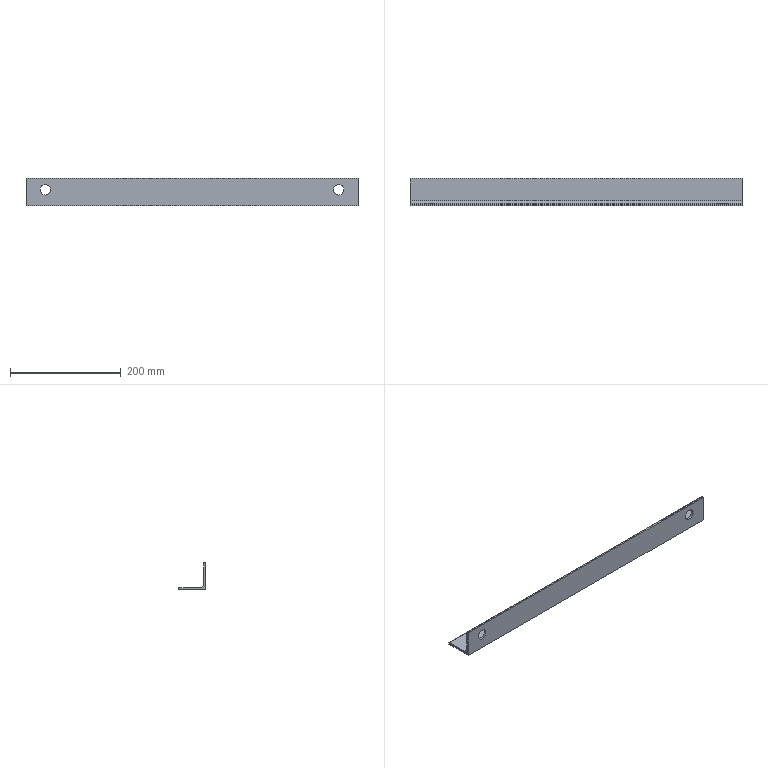Part | STEP file | 计量角钢3_Default<As Machined> | 1 solid | 15 faces | box 598.75 x 50 x 50 mm | volume 231084 mm3 | plane 8 | cylinder 7 | commonest cylinder face diameters 19 x4 2.66 x2 11 x1
STEP:
#1=CARTESIAN_POINT('',(0.,0.,0.));
#2=DIRECTION('',(0.,0.,1.));
#3=DIRECTION('',(1.,0.,0.));
#4=AXIS2_PLACEMENT_3D('',#1,#2,#3);
#5=CARTESIAN_POINT('',(-264.375,0.,38.585));
#6=VERTEX_POINT('',#5);
#7=CARTESIAN_POINT('',(-264.375,4.,38.585));
#8=VERTEX_POINT('',#7);
#9=CARTESIAN_POINT('',(-264.375,-6.,38.585));
#10=DIRECTION('',(0.,1.,0.));
#11=VECTOR('',#10,1.);
#12=LINE('',#9,#11);
#13=CARTESIAN_POINT('',(-264.375,-6.,29.085));
#14=DIRECTION('',(0.,1.,0.));
#15=DIRECTION('',(0.,0.,1.));
#16=AXIS2_PLACEMENT_3D('',#13,#14,#15);
#17=CYLINDRICAL_SURFACE('',#16,9.5);
#18=CARTESIAN_POINT('',(6.283,0.));
#19=DIRECTION('',(0.,1.));
#20=VECTOR('',#19,1.);
#21=LINE('',#18,#20);
#22=(GEOMETRIC_REPRESENTATION_CONTEXT(2)PARAMETRIC_REPRESENTATION_CONTEXT()REPRESENTATION_CONTEXT('',''));
#23=DEFINITIONAL_REPRESENTATION('',(#21),#22);
#24=PCURVE('',#17,#23);
#25=CARTESIAN_POINT('',(-264.375,-6.,29.085));
#26=DIRECTION('',(0.,1.,0.));
#27=DIRECTION('',(0.,0.,1.));
#28=AXIS2_PLACEMENT_3D('',#25,#26,#27);
#29=CYLINDRICAL_SURFACE('',#28,9.5);
#30=CARTESIAN_POINT('',(0.,0.));
#31=DIRECTION('',(0.,1.));
#32=VECTOR('',#31,1.);
#33=LINE('',#30,#32);
#34=(GEOMETRIC_REPRESENTATION_CONTEXT(2)PARAMETRIC_REPRESENTATION_CONTEXT()REPRESENTATION_CONTEXT('',''));
#35=DEFINITIONAL_REPRESENTATION('',(#33),#34);
#36=PCURVE('',#29,#35);
#37=SURFACE_CURVE('',#12,(#24,#36),.PCURVE_S1.);
#38=EDGE_CURVE('',#6,#8,#37,.T.);
#39=ORIENTED_EDGE('',*,*,#38,.T.);
#40=CARTESIAN_POINT('',(-264.375,4.,19.585));
#41=VERTEX_POINT('',#40);
#42=CARTESIAN_POINT('',(-264.375,4.,29.085));
#43=DIRECTION('',(0.,1.,0.));
#44=DIRECTION('',(0.,0.,1.));
#45=AXIS2_PLACEMENT_3D('',#42,#43,#44);
#46=CIRCLE('',#45,9.5);
#47=CARTESIAN_POINT('',(0.,10.));
#48=DIRECTION('',(1.,0.));
#49=VECTOR('',#48,1.);
#50=LINE('',#47,#49);
#51=(GEOMETRIC_REPRESENTATION_CONTEXT(2)PARAMETRIC_REPRESENTATION_CONTEXT()REPRESENTATION_CONTEXT('',''));
#52=DEFINITIONAL_REPRESENTATION('',(#50),#51);
#53=PCURVE('',#17,#52);
#54=CARTESIAN_POINT('',(299.375,4.,48.67));
#55=DIRECTION('',(0.,-1.,0.));
#56=DIRECTION('',(1.,0.,0.));
#57=AXIS2_PLACEMENT_3D('',#54,#55,#56);
#58=PLANE('',#57);
#59=CARTESIAN_POINT('',(-563.75,-10.085));
#60=CARTESIAN_POINT('',(-547.296,-10.085));
#61=CARTESIAN_POINT('',(-555.523,-24.335));
#62=CARTESIAN_POINT('',(-563.75,-38.585));
#63=CARTESIAN_POINT('',(-571.977,-24.335));
#64=CARTESIAN_POINT('',(-580.204,-10.085));
#65=CARTESIAN_POINT('',(-563.75,-10.085));
#66=(BOUNDED_CURVE()B_SPLINE_CURVE(2,(#59,#60,#61,#62,#63,#64,#65),.UNSPECIFIED.,.T.,.F.)B_SPLINE_CURVE_WITH_KNOTS((1,2,2,2,2,1),(-2.094,0.,2.094,4.189,6.283,8.378),.UNSPECIFIED.)CURVE()GEOMETRIC_REPRESENTATION_ITEM()RATIONAL_B_SPLINE_CURVE((1.,0.5,1.,0.5,1.,0.5,1.))REPRESENTATION_ITEM(''));
#67=(GEOMETRIC_REPRESENTATION_CONTEXT(2)PARAMETRIC_REPRESENTATION_CONTEXT()REPRESENTATION_CONTEXT('',''));
#68=DEFINITIONAL_REPRESENTATION('',(#66),#67);
#69=PCURVE('',#58,#68);
#70=SURFACE_CURVE('',#46,(#53,#69),.PCURVE_S1.);
#71=EDGE_CURVE('',#41,#8,#70,.T.);
#72=ORIENTED_EDGE('',*,*,#71,.F.);
#73=CARTESIAN_POINT('',(-264.375,0.,19.585));
#74=VERTEX_POINT('',#73);
#75=CARTESIAN_POINT('',(-264.375,-6.,19.585));
#76=DIRECTION('',(0.,1.,0.));
#77=VECTOR('',#76,1.);
#78=LINE('',#75,#77);
#79=CARTESIAN_POINT('',(3.142,0.));
#80=DIRECTION('',(0.,1.));
#81=VECTOR('',#80,1.);
#82=LINE('',#79,#81);
#83=(GEOMETRIC_REPRESENTATION_CONTEXT(2)PARAMETRIC_REPRESENTATION_CONTEXT()REPRESENTATION_CONTEXT('',''));
#84=DEFINITIONAL_REPRESENTATION('',(#82),#83);
#85=PCURVE('',#17,#84);
#86=CARTESIAN_POINT('',(3.142,0.));
#87=DIRECTION('',(0.,1.));
#88=VECTOR('',#87,1.);
#89=LINE('',#86,#88);
#90=(GEOMETRIC_REPRESENTATION_CONTEXT(2)PARAMETRIC_REPRESENTATION_CONTEXT()REPRESENTATION_CONTEXT('',''));
#91=DEFINITIONAL_REPRESENTATION('',(#89),#90);
#92=PCURVE('',#29,#91);
#93=SURFACE_CURVE('',#78,(#85,#92),.PCURVE_S1.);
#94=EDGE_CURVE('',#74,#41,#93,.T.);
#95=ORIENTED_EDGE('',*,*,#94,.F.);
#96=CARTESIAN_POINT('',(-264.375,0.,29.085));
#97=DIRECTION('',(0.,1.,0.));
#98=DIRECTION('',(-1.,0.,0.));
#99=AXIS2_PLACEMENT_3D('',#96,#97,#98);
#100=CIRCLE('',#99,9.5);
#101=CARTESIAN_POINT('',(-1.571,6.));
#102=DIRECTION('',(1.,0.));
#103=VECTOR('',#102,1.);
#104=LINE('',#101,#103);
#105=(GEOMETRIC_REPRESENTATION_CONTEXT(2)PARAMETRIC_REPRESENTATION_CONTEXT()REPRESENTATION_CONTEXT('',''));
#106=DEFINITIONAL_REPRESENTATION('',(#104),#105);
#107=PCURVE('',#17,#106);
#108=CARTESIAN_POINT('',(299.375,0.,50.));
#109=DIRECTION('',(0.,1.,0.));
#110=DIRECTION('',(-1.,0.,0.));
#111=AXIS2_PLACEMENT_3D('',#108,#109,#110);
#112=PLANE('',#111);
#113=CARTESIAN_POINT('',(563.75,-20.915));
#114=DIRECTION('',(1.,0.));
#115=AXIS2_PLACEMENT_2D('',#113,#114);
#116=CIRCLE('',#115,9.5);
#117=(GEOMETRIC_REPRESENTATION_CONTEXT(2)PARAMETRIC_REPRESENTATION_CONTEXT()REPRESENTATION_CONTEXT('',''));
#118=DEFINITIONAL_REPRESENTATION('',(#116),#117);
#119=PCURVE('',#112,#118);
#120=SURFACE_CURVE('',#100,(#107,#119),.PCURVE_S1.);
#121=EDGE_CURVE('',#74,#6,#120,.T.);
#122=ORIENTED_EDGE('',*,*,#121,.T.);
#123=EDGE_LOOP('',(#39,#72,#95,#122));
#124=FACE_BOUND('',#123,.F.);
#125=ADVANCED_FACE('',(#124),#17,.F.);
#126=CARTESIAN_POINT('',(264.375,0.,38.585));
#127=VERTEX_POINT('',#126);
#128=CARTESIAN_POINT('',(264.375,4.,38.585));
#129=VERTEX_POINT('',#128);
#130=CARTESIAN_POINT('',(264.375,-6.,38.585));
#131=DIRECTION('',(0.,1.,0.));
#132=VECTOR('',#131,1.);
#133=LINE('',#130,#132);
#134=CARTESIAN_POINT('',(264.375,-6.,29.085));
#135=DIRECTION('',(0.,1.,0.));
#136=DIRECTION('',(0.,0.,1.));
#137=AXIS2_PLACEMENT_3D('',#134,#135,#136);
#138=CYLINDRICAL_SURFACE('',#137,9.5);
#139=CARTESIAN_POINT('',(6.283,0.));
#140=DIRECTION('',(0.,1.));
#141=VECTOR('',#140,1.);
#142=LINE('',#139,#141);
#143=(GEOMETRIC_REPRESENTATION_CONTEXT(2)PARAMETRIC_REPRESENTATION_CONTEXT()REPRESENTATION_CONTEXT('',''));
#144=DEFINITIONAL_REPRESENTATION('',(#142),#143);
#145=PCURVE('',#138,#144);
#146=CARTESIAN_POINT('',(264.375,-6.,29.085));
#147=DIRECTION('',(0.,1.,0.));
#148=DIRECTION('',(0.,0.,1.));
#149=AXIS2_PLACEMENT_3D('',#146,#147,#148);
#150=CYLINDRICAL_SURFACE('',#149,9.5);
#151=CARTESIAN_POINT('',(0.,0.));
#152=DIRECTION('',(0.,1.));
#153=VECTOR('',#152,1.);
#154=LINE('',#151,#153);
#155=(GEOMETRIC_REPRESENTATION_CONTEXT(2)PARAMETRIC_REPRESENTATION_CONTEXT()REPRESENTATION_CONTEXT('',''));
#156=DEFINITIONAL_REPRESENTATION('',(#154),#155);
#157=PCURVE('',#150,#156);
#158=SURFACE_CURVE('',#133,(#145,#157),.PCURVE_S1.);
#159=EDGE_CURVE('',#127,#129,#158,.T.);
#160=ORIENTED_EDGE('',*,*,#159,.T.);
#161=CARTESIAN_POINT('',(264.375,4.,19.585));
#162=VERTEX_POINT('',#161);
#163=CARTESIAN_POINT('',(264.375,4.,29.085));
#164=DIRECTION('',(0.,1.,0.));
#165=DIRECTION('',(0.,0.,-1.));
#166=AXIS2_PLACEMENT_3D('',#163,#164,#165);
#167=CIRCLE('',#166,9.5);
#168=CARTESIAN_POINT('',(3.142,10.));
#169=DIRECTION('',(1.,0.));
#170=VECTOR('',#169,1.);
#171=LINE('',#168,#170);
#172=(GEOMETRIC_REPRESENTATION_CONTEXT(2)PARAMETRIC_REPRESENTATION_CONTEXT()REPRESENTATION_CONTEXT('',''));
#173=DEFINITIONAL_REPRESENTATION('',(#171),#172);
#174=PCURVE('',#138,#173);
#175=CARTESIAN_POINT('',(-35.,-29.085));
#176=CARTESIAN_POINT('',(-51.454,-29.085));
#177=CARTESIAN_POINT('',(-43.227,-14.835));
#178=CARTESIAN_POINT('',(-35.,-0.585));
#179=CARTESIAN_POINT('',(-26.773,-14.835));
#180=CARTESIAN_POINT('',(-18.546,-29.085));
#181=CARTESIAN_POINT('',(-35.,-29.085));
#182=(BOUNDED_CURVE()B_SPLINE_CURVE(2,(#175,#176,#177,#178,#179,#180,#181),.UNSPECIFIED.,.T.,.F.)B_SPLINE_CURVE_WITH_KNOTS((1,2,2,2,2,1),(-2.094,0.,2.094,4.189,6.283,8.378),.UNSPECIFIED.)CURVE()GEOMETRIC_REPRESENTATION_ITEM()RATIONAL_B_SPLINE_CURVE((1.,0.5,1.,0.5,1.,0.5,1.))REPRESENTATION_ITEM(''));
#183=(GEOMETRIC_REPRESENTATION_CONTEXT(2)PARAMETRIC_REPRESENTATION_CONTEXT()REPRESENTATION_CONTEXT('',''));
#184=DEFINITIONAL_REPRESENTATION('',(#182),#183);
#185=PCURVE('',#58,#184);
#186=SURFACE_CURVE('',#167,(#174,#185),.PCURVE_S1.);
#187=EDGE_CURVE('',#162,#129,#186,.T.);
#188=ORIENTED_EDGE('',*,*,#187,.F.);
#189=CARTESIAN_POINT('',(264.375,0.,19.585));
#190=VERTEX_POINT('',#189);
#191=CARTESIAN_POINT('',(264.375,-6.,19.585));
#192=DIRECTION('',(0.,1.,0.));
#193=VECTOR('',#192,1.);
#194=LINE('',#191,#193);
#195=CARTESIAN_POINT('',(3.142,0.));
#196=DIRECTION('',(0.,1.));
#197=VECTOR('',#196,1.);
#198=LINE('',#195,#197);
#199=(GEOMETRIC_REPRESENTATION_CONTEXT(2)PARAMETRIC_REPRESENTATION_CONTEXT()REPRESENTATION_CONTEXT('',''));
#200=DEFINITIONAL_REPRESENTATION('',(#198),#199);
#201=PCURVE('',#138,#200);
#202=CARTESIAN_POINT('',(3.142,0.));
#203=DIRECTION('',(0.,1.));
#204=VECTOR('',#203,1.);
#205=LINE('',#202,#204);
#206=(GEOMETRIC_REPRESENTATION_CONTEXT(2)PARAMETRIC_REPRESENTATION_CONTEXT()REPRESENTATION_CONTEXT('',''));
#207=DEFINITIONAL_REPRESENTATION('',(#205),#206);
#208=PCURVE('',#150,#207);
#209=SURFACE_CURVE('',#194,(#201,#208),.PCURVE_S1.);
#210=EDGE_CURVE('',#190,#162,#209,.T.);
#211=ORIENTED_EDGE('',*,*,#210,.F.);
#212=CARTESIAN_POINT('',(264.375,0.,29.085));
#213=DIRECTION('',(0.,1.,0.));
#214=DIRECTION('',(-1.,0.,0.));
#215=AXIS2_PLACEMENT_3D('',#212,#213,#214);
#216=CIRCLE('',#215,9.5);
#217=CARTESIAN_POINT('',(-1.571,6.));
#218=DIRECTION('',(1.,0.));
#219=VECTOR('',#218,1.);
#220=LINE('',#217,#219);
#221=(GEOMETRIC_REPRESENTATION_CONTEXT(2)PARAMETRIC_REPRESENTATION_CONTEXT()REPRESENTATION_CONTEXT('',''));
#222=DEFINITIONAL_REPRESENTATION('',(#220),#221);
#223=PCURVE('',#138,#222);
#224=CARTESIAN_POINT('',(35.,-20.915));
#225=DIRECTION('',(1.,0.));
#226=AXIS2_PLACEMENT_2D('',#224,#225);
#227=CIRCLE('',#226,9.5);
#228=(GEOMETRIC_REPRESENTATION_CONTEXT(2)PARAMETRIC_REPRESENTATION_CONTEXT()REPRESENTATION_CONTEXT('',''));
#229=DEFINITIONAL_REPRESENTATION('',(#227),#228);
#230=PCURVE('',#112,#229);
#231=SURFACE_CURVE('',#216,(#223,#230),.PCURVE_S1.);
#232=EDGE_CURVE('',#190,#127,#231,.T.);
#233=ORIENTED_EDGE('',*,*,#232,.T.);
#234=EDGE_LOOP('',(#160,#188,#211,#233));
#235=FACE_BOUND('',#234,.F.);
#236=ADVANCED_FACE('',(#235),#138,.F.);
#237=CARTESIAN_POINT('',(-299.375,50.,2.67));
#238=VERTEX_POINT('',#237);
#239=CARTESIAN_POINT('',(-299.375,48.67,4.));
#240=VERTEX_POINT('',#239);
#241=CARTESIAN_POINT('',(-299.375,48.67,2.67));
#242=DIRECTION('',(1.,0.,0.));
#243=DIRECTION('',(0.,1.,0.));
#244=AXIS2_PLACEMENT_3D('',#241,#242,#243);
#245=CIRCLE('',#244,1.33);
#246=CARTESIAN_POINT('',(299.375,48.67,2.67));
#247=DIRECTION('',(-1.,0.,0.));
#248=DIRECTION('',(0.,-1.,0.));
#249=AXIS2_PLACEMENT_3D('',#246,#247,#248);
#250=CYLINDRICAL_SURFACE('',#249,1.33);
#251=CARTESIAN_POINT('',(3.142,598.75));
#252=DIRECTION('',(-1.,0.));
#253=VECTOR('',#252,1.);
#254=LINE('',#251,#253);
#255=(GEOMETRIC_REPRESENTATION_CONTEXT(2)PARAMETRIC_REPRESENTATION_CONTEXT()REPRESENTATION_CONTEXT('',''));
#256=DEFINITIONAL_REPRESENTATION('',(#254),#255);
#257=PCURVE('',#250,#256);
#258=CARTESIAN_POINT('',(-299.375,48.67,2.67));
#259=DIRECTION('',(1.,0.,0.));
#260=DIRECTION('',(0.,1.,0.));
#261=AXIS2_PLACEMENT_3D('',#258,#259,#260);
#262=PLANE('',#261);
#263=CARTESIAN_POINT('',(0.,0.));
#264=DIRECTION('',(1.,0.));
#265=AXIS2_PLACEMENT_2D('',#263,#264);
#266=CIRCLE('',#265,1.33);
#267=(GEOMETRIC_REPRESENTATION_CONTEXT(2)PARAMETRIC_REPRESENTATION_CONTEXT()REPRESENTATION_CONTEXT('',''));
#268=DEFINITIONAL_REPRESENTATION('',(#266),#267);
#269=PCURVE('',#262,#268);
#270=SURFACE_CURVE('',#245,(#257,#269),.PCURVE_S1.);
#271=EDGE_CURVE('',#238,#240,#270,.T.);
#272=ORIENTED_EDGE('',*,*,#271,.T.);
#273=CARTESIAN_POINT('',(299.375,48.67,4.));
#274=VERTEX_POINT('',#273);
#275=CARTESIAN_POINT('',(299.375,48.67,4.));
#276=DIRECTION('',(-1.,0.,0.));
#277=VECTOR('',#276,1.);
#278=LINE('',#275,#277);
#279=CARTESIAN_POINT('',(1.571,0.));
#280=DIRECTION('',(0.,1.));
#281=VECTOR('',#280,1.);
#282=LINE('',#279,#281);
#283=(GEOMETRIC_REPRESENTATION_CONTEXT(2)PARAMETRIC_REPRESENTATION_CONTEXT()REPRESENTATION_CONTEXT('',''));
#284=DEFINITIONAL_REPRESENTATION('',(#282),#283);
#285=PCURVE('',#250,#284);
#286=CARTESIAN_POINT('',(299.375,9.5,4.));
#287=DIRECTION('',(0.,0.,-1.));
#288=DIRECTION('',(-1.,0.,0.));
#289=AXIS2_PLACEMENT_3D('',#286,#287,#288);
#290=PLANE('',#289);
#291=CARTESIAN_POINT('',(0.,39.17));
#292=DIRECTION('',(1.,0.));
#293=VECTOR('',#292,1.);
#294=LINE('',#291,#293);
#295=(GEOMETRIC_REPRESENTATION_CONTEXT(2)PARAMETRIC_REPRESENTATION_CONTEXT()REPRESENTATION_CONTEXT('',''));
#296=DEFINITIONAL_REPRESENTATION('',(#294),#295);
#297=PCURVE('',#290,#296);
#298=SURFACE_CURVE('',#278,(#285,#297),.PCURVE_S1.);
#299=EDGE_CURVE('',#274,#240,#298,.T.);
#300=ORIENTED_EDGE('',*,*,#299,.F.);
#301=CARTESIAN_POINT('',(299.375,50.,2.67));
#302=VERTEX_POINT('',#301);
#303=CARTESIAN_POINT('',(299.375,48.67,2.67));
#304=DIRECTION('',(1.,0.,0.));
#305=DIRECTION('',(0.,1.,0.));
#306=AXIS2_PLACEMENT_3D('',#303,#304,#305);
#307=CIRCLE('',#306,1.33);
#308=CARTESIAN_POINT('',(3.142,0.));
#309=DIRECTION('',(-1.,0.));
#310=VECTOR('',#309,1.);
#311=LINE('',#308,#310);
#312=(GEOMETRIC_REPRESENTATION_CONTEXT(2)PARAMETRIC_REPRESENTATION_CONTEXT()REPRESENTATION_CONTEXT('',''));
#313=DEFINITIONAL_REPRESENTATION('',(#311),#312);
#314=PCURVE('',#250,#313);
#315=CARTESIAN_POINT('',(299.375,48.67,2.67));
#316=DIRECTION('',(1.,0.,0.));
#317=DIRECTION('',(0.,1.,0.));
#318=AXIS2_PLACEMENT_3D('',#315,#316,#317);
#319=PLANE('',#318);
#320=CARTESIAN_POINT('',(0.,0.));
#321=DIRECTION('',(1.,0.));
#322=AXIS2_PLACEMENT_2D('',#320,#321);
#323=CIRCLE('',#322,1.33);
#324=(GEOMETRIC_REPRESENTATION_CONTEXT(2)PARAMETRIC_REPRESENTATION_CONTEXT()REPRESENTATION_CONTEXT('',''));
#325=DEFINITIONAL_REPRESENTATION('',(#323),#324);
#326=PCURVE('',#319,#325);
#327=SURFACE_CURVE('',#307,(#314,#326),.PCURVE_S1.);
#328=EDGE_CURVE('',#302,#274,#327,.T.);
#329=ORIENTED_EDGE('',*,*,#328,.F.);
#330=CARTESIAN_POINT('',(299.375,50.,2.67));
#331=DIRECTION('',(-1.,0.,0.));
#332=VECTOR('',#331,1.);
#333=LINE('',#330,#332);
#334=CARTESIAN_POINT('',(3.142,0.));
#335=DIRECTION('',(0.,1.));
#336=VECTOR('',#335,1.);
#337=LINE('',#334,#336);
#338=(GEOMETRIC_REPRESENTATION_CONTEXT(2)PARAMETRIC_REPRESENTATION_CONTEXT()REPRESENTATION_CONTEXT('',''));
#339=DEFINITIONAL_REPRESENTATION('',(#337),#338);
#340=PCURVE('',#250,#339);
#341=CARTESIAN_POINT('',(299.375,50.,2.67));
#342=DIRECTION('',(0.,-1.,0.));
#343=DIRECTION('',(1.,0.,0.));
#344=AXIS2_PLACEMENT_3D('',#341,#342,#343);
#345=PLANE('',#344);
#346=CARTESIAN_POINT('',(0.,0.));
#347=DIRECTION('',(-1.,0.));
#348=VECTOR('',#347,1.);
#349=LINE('',#346,#348);
#350=(GEOMETRIC_REPRESENTATION_CONTEXT(2)PARAMETRIC_REPRESENTATION_CONTEXT()REPRESENTATION_CONTEXT('',''));
#351=DEFINITIONAL_REPRESENTATION('',(#349),#350);
#352=PCURVE('',#345,#351);
#353=SURFACE_CURVE('',#333,(#340,#352),.PCURVE_S1.);
#354=EDGE_CURVE('',#302,#238,#353,.T.);
#355=ORIENTED_EDGE('',*,*,#354,.T.);
#356=EDGE_LOOP('',(#272,#300,#329,#355));
#357=FACE_BOUND('',#356,.T.);
#358=ADVANCED_FACE('',(#357),#250,.T.);
#359=CARTESIAN_POINT('',(-299.375,9.5,4.));
#360=VERTEX_POINT('',#359);
#361=CARTESIAN_POINT('',(-299.375,9.5,4.));
#362=DIRECTION('',(0.,-1.,0.));
#363=VECTOR('',#362,1.);
#364=LINE('',#361,#363);
#365=CARTESIAN_POINT('',(598.75,0.));
#366=DIRECTION('',(0.,-1.));
#367=VECTOR('',#366,1.);
#368=LINE('',#365,#367);
#369=(GEOMETRIC_REPRESENTATION_CONTEXT(2)PARAMETRIC_REPRESENTATION_CONTEXT()REPRESENTATION_CONTEXT('',''));
#370=DEFINITIONAL_REPRESENTATION('',(#368),#369);
#371=PCURVE('',#290,#370);
#372=CARTESIAN_POINT('',(-39.17,1.33));
#373=DIRECTION('',(-1.,0.));
#374=VECTOR('',#373,1.);
#375=LINE('',#372,#374);
#376=(GEOMETRIC_REPRESENTATION_CONTEXT(2)PARAMETRIC_REPRESENTATION_CONTEXT()REPRESENTATION_CONTEXT('',''));
#377=DEFINITIONAL_REPRESENTATION('',(#375),#376);
#378=PCURVE('',#262,#377);
#379=SURFACE_CURVE('',#364,(#371,#378),.PCURVE_S1.);
#380=EDGE_CURVE('',#240,#360,#379,.T.);
#381=ORIENTED_EDGE('',*,*,#380,.T.);
#382=CARTESIAN_POINT('',(299.375,9.5,4.));
#383=VERTEX_POINT('',#382);
#384=CARTESIAN_POINT('',(299.375,9.5,4.));
#385=DIRECTION('',(-1.,0.,0.));
#386=VECTOR('',#385,1.);
#387=LINE('',#384,#386);
#388=CARTESIAN_POINT('',(0.,0.));
#389=DIRECTION('',(1.,0.));
#390=VECTOR('',#389,1.);
#391=LINE('',#388,#390);
#392=(GEOMETRIC_REPRESENTATION_CONTEXT(2)PARAMETRIC_REPRESENTATION_CONTEXT()REPRESENTATION_CONTEXT('',''));
#393=DEFINITIONAL_REPRESENTATION('',(#391),#392);
#394=PCURVE('',#290,#393);
#395=CARTESIAN_POINT('',(299.375,9.5,9.5));
#396=DIRECTION('',(-1.,0.,0.));
#397=DIRECTION('',(0.,-1.,0.));
#398=AXIS2_PLACEMENT_3D('',#395,#396,#397);
#399=CYLINDRICAL_SURFACE('',#398,5.5);
#400=CARTESIAN_POINT('',(4.712,0.));
#401=DIRECTION('',(0.,1.));
#402=VECTOR('',#401,1.);
#403=LINE('',#400,#402);
#404=(GEOMETRIC_REPRESENTATION_CONTEXT(2)PARAMETRIC_REPRESENTATION_CONTEXT()REPRESENTATION_CONTEXT('',''));
#405=DEFINITIONAL_REPRESENTATION('',(#403),#404);
#406=PCURVE('',#399,#405);
#407=SURFACE_CURVE('',#387,(#394,#406),.PCURVE_S1.);
#408=EDGE_CURVE('',#383,#360,#407,.T.);
#409=ORIENTED_EDGE('',*,*,#408,.F.);
#410=CARTESIAN_POINT('',(299.375,9.5,4.));
#411=DIRECTION('',(0.,-1.,0.));
#412=VECTOR('',#411,1.);
#413=LINE('',#410,#412);
#414=CARTESIAN_POINT('',(0.,0.));
#415=DIRECTION('',(0.,-1.));
#416=VECTOR('',#415,1.);
#417=LINE('',#414,#416);
#418=(GEOMETRIC_REPRESENTATION_CONTEXT(2)PARAMETRIC_REPRESENTATION_CONTEXT()REPRESENTATION_CONTEXT('',''));
#419=DEFINITIONAL_REPRESENTATION('',(#417),#418);
#420=PCURVE('',#290,#419);
#421=CARTESIAN_POINT('',(-39.17,1.33));
#422=DIRECTION('',(-1.,0.));
#423=VECTOR('',#422,1.);
#424=LINE('',#421,#423);
#425=(GEOMETRIC_REPRESENTATION_CONTEXT(2)PARAMETRIC_REPRESENTATION_CONTEXT()REPRESENTATION_CONTEXT('',''));
#426=DEFINITIONAL_REPRESENTATION('',(#424),#425);
#427=PCURVE('',#319,#426);
#428=SURFACE_CURVE('',#413,(#420,#427),.PCURVE_S1.);
#429=EDGE_CURVE('',#274,#383,#428,.T.);
#430=ORIENTED_EDGE('',*,*,#429,.F.);
#431=ORIENTED_EDGE('',*,*,#299,.T.);
#432=EDGE_LOOP('',(#381,#409,#430,#431));
#433=FACE_BOUND('',#432,.T.);
#434=ADVANCED_FACE('',(#433),#290,.F.);
#435=ORIENTED_EDGE('',*,*,#408,.F.);
#436=CARTESIAN_POINT('',(299.375,4.,9.5));
#437=VERTEX_POINT('',#436);
#438=CARTESIAN_POINT('',(299.375,9.5,9.5));
#439=DIRECTION('',(-1.,0.,0.));
#440=DIRECTION('',(0.,1.,0.));
#441=AXIS2_PLACEMENT_3D('',#438,#439,#440);
#442=CIRCLE('',#441,5.5);
#443=CARTESIAN_POINT('',(3.142,0.));
#444=DIRECTION('',(1.,0.));
#445=VECTOR('',#444,1.);
#446=LINE('',#443,#445);
#447=(GEOMETRIC_REPRESENTATION_CONTEXT(2)PARAMETRIC_REPRESENTATION_CONTEXT()REPRESENTATION_CONTEXT('',''));
#448=DEFINITIONAL_REPRESENTATION('',(#446),#447);
#449=PCURVE('',#399,#448);
#450=CARTESIAN_POINT('',(-33.67,6.83));
#451=CARTESIAN_POINT('',(-33.67,-2.696));
#452=CARTESIAN_POINT('',(-41.92,2.067));
#453=CARTESIAN_POINT('',(-50.17,6.83));
#454=CARTESIAN_POINT('',(-41.92,11.593));
#455=CARTESIAN_POINT('',(-33.67,16.356));
#456=CARTESIAN_POINT('',(-33.67,6.83));
#457=(BOUNDED_CURVE()B_SPLINE_CURVE(2,(#450,#451,#452,#453,#454,#455,#456),.UNSPECIFIED.,.T.,.F.)B_SPLINE_CURVE_WITH_KNOTS((1,2,2,2,2,1),(-2.094,0.,2.094,4.189,6.283,8.378),.UNSPECIFIED.)CURVE()GEOMETRIC_REPRESENTATION_ITEM()RATIONAL_B_SPLINE_CURVE((1.,0.5,1.,0.5,1.,0.5,1.))REPRESENTATION_ITEM(''));
#458=(GEOMETRIC_REPRESENTATION_CONTEXT(2)PARAMETRIC_REPRESENTATION_CONTEXT()REPRESENTATION_CONTEXT('',''));
#459=DEFINITIONAL_REPRESENTATION('',(#457),#458);
#460=PCURVE('',#319,#459);
#461=SURFACE_CURVE('',#442,(#449,#460),.PCURVE_S1.);
#462=EDGE_CURVE('',#383,#437,#461,.T.);
#463=ORIENTED_EDGE('',*,*,#462,.T.);
#464=CARTESIAN_POINT('',(-299.375,4.,9.5));
#465=VERTEX_POINT('',#464);
#466=CARTESIAN_POINT('',(299.375,4.,9.5));
#467=DIRECTION('',(-1.,0.,0.));
#468=VECTOR('',#467,1.);
#469=LINE('',#466,#468);
#470=CARTESIAN_POINT('',(6.283,0.));
#471=DIRECTION('',(0.,1.));
#472=VECTOR('',#471,1.);
#473=LINE('',#470,#472);
#474=(GEOMETRIC_REPRESENTATION_CONTEXT(2)PARAMETRIC_REPRESENTATION_CONTEXT()REPRESENTATION_CONTEXT('',''));
#475=DEFINITIONAL_REPRESENTATION('',(#473),#474);
#476=PCURVE('',#399,#475);
#477=CARTESIAN_POINT('',(0.,-39.17));
#478=DIRECTION('',(-1.,0.));
#479=VECTOR('',#478,1.);
#480=LINE('',#477,#479);
#481=(GEOMETRIC_REPRESENTATION_CONTEXT(2)PARAMETRIC_REPRESENTATION_CONTEXT()REPRESENTATION_CONTEXT('',''));
#482=DEFINITIONAL_REPRESENTATION('',(#480),#481);
#483=PCURVE('',#58,#482);
#484=SURFACE_CURVE('',#469,(#476,#483),.PCURVE_S1.);
#485=EDGE_CURVE('',#437,#465,#484,.T.);
#486=ORIENTED_EDGE('',*,*,#485,.T.);
#487=CARTESIAN_POINT('',(-299.375,9.5,9.5));
#488=DIRECTION('',(-1.,0.,0.));
#489=DIRECTION('',(0.,1.,0.));
#490=AXIS2_PLACEMENT_3D('',#487,#488,#489);
#491=CIRCLE('',#490,5.5);
#492=CARTESIAN_POINT('',(3.142,598.75));
#493=DIRECTION('',(1.,0.));
#494=VECTOR('',#493,1.);
#495=LINE('',#492,#494);
#496=(GEOMETRIC_REPRESENTATION_CONTEXT(2)PARAMETRIC_REPRESENTATION_CONTEXT()REPRESENTATION_CONTEXT('',''));
#497=DEFINITIONAL_REPRESENTATION('',(#495),#496);
#498=PCURVE('',#399,#497);
#499=CARTESIAN_POINT('',(-33.67,6.83));
#500=CARTESIAN_POINT('',(-33.67,-2.696));
#501=CARTESIAN_POINT('',(-41.92,2.067));
#502=CARTESIAN_POINT('',(-50.17,6.83));
#503=CARTESIAN_POINT('',(-41.92,11.593));
#504=CARTESIAN_POINT('',(-33.67,16.356));
#505=CARTESIAN_POINT('',(-33.67,6.83));
#506=(BOUNDED_CURVE()B_SPLINE_CURVE(2,(#499,#500,#501,#502,#503,#504,#505),.UNSPECIFIED.,.T.,.F.)B_SPLINE_CURVE_WITH_KNOTS((1,2,2,2,2,1),(-2.094,0.,2.094,4.189,6.283,8.378),.UNSPECIFIED.)CURVE()GEOMETRIC_REPRESENTATION_ITEM()RATIONAL_B_SPLINE_CURVE((1.,0.5,1.,0.5,1.,0.5,1.))REPRESENTATION_ITEM(''));
#507=(GEOMETRIC_REPRESENTATION_CONTEXT(2)PARAMETRIC_REPRESENTATION_CONTEXT()REPRESENTATION_CONTEXT('',''));
#508=DEFINITIONAL_REPRESENTATION('',(#506),#507);
#509=PCURVE('',#262,#508);
#510=SURFACE_CURVE('',#491,(#498,#509),.PCURVE_S1.);
#511=EDGE_CURVE('',#360,#465,#510,.T.);
#512=ORIENTED_EDGE('',*,*,#511,.F.);
#513=EDGE_LOOP('',(#435,#463,#486,#512));
#514=FACE_BOUND('',#513,.F.);
#515=ADVANCED_FACE('',(#514),#399,.F.);
#516=CARTESIAN_POINT('',(-264.375,4.,29.085));
#517=DIRECTION('',(0.,1.,0.));
#518=DIRECTION('',(0.,0.,1.));
#519=AXIS2_PLACEMENT_3D('',#516,#517,#518);
#520=CIRCLE('',#519,9.5);
#521=CARTESIAN_POINT('',(-563.75,-10.085));
#522=CARTESIAN_POINT('',(-547.296,-10.085));
#523=CARTESIAN_POINT('',(-555.523,-24.335));
#524=CARTESIAN_POINT('',(-563.75,-38.585));
#525=CARTESIAN_POINT('',(-571.977,-24.335));
#526=CARTESIAN_POINT('',(-580.204,-10.085));
#527=CARTESIAN_POINT('',(-563.75,-10.085));
#528=(BOUNDED_CURVE()B_SPLINE_CURVE(2,(#521,#522,#523,#524,#525,#526,#527),.UNSPECIFIED.,.T.,.F.)B_SPLINE_CURVE_WITH_KNOTS((1,2,2,2,2,1),(-2.094,0.,2.094,4.189,6.283,8.378),.UNSPECIFIED.)CURVE()GEOMETRIC_REPRESENTATION_ITEM()RATIONAL_B_SPLINE_CURVE((1.,0.5,1.,0.5,1.,0.5,1.))REPRESENTATION_ITEM(''));
#529=(GEOMETRIC_REPRESENTATION_CONTEXT(2)PARAMETRIC_REPRESENTATION_CONTEXT()REPRESENTATION_CONTEXT('',''));
#530=DEFINITIONAL_REPRESENTATION('',(#528),#529);
#531=PCURVE('',#58,#530);
#532=CARTESIAN_POINT('',(0.,10.));
#533=DIRECTION('',(1.,0.));
#534=VECTOR('',#533,1.);
#535=LINE('',#532,#534);
#536=(GEOMETRIC_REPRESENTATION_CONTEXT(2)PARAMETRIC_REPRESENTATION_CONTEXT()REPRESENTATION_CONTEXT('',''));
#537=DEFINITIONAL_REPRESENTATION('',(#535),#536);
#538=PCURVE('',#29,#537);
#539=SURFACE_CURVE('',#520,(#531,#538),.PCURVE_S1.);
#540=EDGE_CURVE('',#8,#41,#539,.T.);
#541=ORIENTED_EDGE('',*,*,#540,.F.);
#542=ORIENTED_EDGE('',*,*,#71,.F.);
#543=EDGE_LOOP('',(#541,#542));
#544=FACE_BOUND('',#543,.T.);
#545=CARTESIAN_POINT('',(264.375,4.,29.085));
#546=DIRECTION('',(0.,1.,0.));
#547=DIRECTION('',(0.,0.,-1.));
#548=AXIS2_PLACEMENT_3D('',#545,#546,#547);
#549=CIRCLE('',#548,9.5);
#550=CARTESIAN_POINT('',(-35.,-29.085));
#551=CARTESIAN_POINT('',(-51.454,-29.085));
#552=CARTESIAN_POINT('',(-43.227,-14.835));
#553=CARTESIAN_POINT('',(-35.,-0.585));
#554=CARTESIAN_POINT('',(-26.773,-14.835));
#555=CARTESIAN_POINT('',(-18.546,-29.085));
#556=CARTESIAN_POINT('',(-35.,-29.085));
#557=(BOUNDED_CURVE()B_SPLINE_CURVE(2,(#550,#551,#552,#553,#554,#555,#556),.UNSPECIFIED.,.T.,.F.)B_SPLINE_CURVE_WITH_KNOTS((1,2,2,2,2,1),(-2.094,0.,2.094,4.189,6.283,8.378),.UNSPECIFIED.)CURVE()GEOMETRIC_REPRESENTATION_ITEM()RATIONAL_B_SPLINE_CURVE((1.,0.5,1.,0.5,1.,0.5,1.))REPRESENTATION_ITEM(''));
#558=(GEOMETRIC_REPRESENTATION_CONTEXT(2)PARAMETRIC_REPRESENTATION_CONTEXT()REPRESENTATION_CONTEXT('',''));
#559=DEFINITIONAL_REPRESENTATION('',(#557),#558);
#560=PCURVE('',#58,#559);
#561=CARTESIAN_POINT('',(-3.142,10.));
#562=DIRECTION('',(1.,0.));
#563=VECTOR('',#562,1.);
#564=LINE('',#561,#563);
#565=(GEOMETRIC_REPRESENTATION_CONTEXT(2)PARAMETRIC_REPRESENTATION_CONTEXT()REPRESENTATION_CONTEXT('',''));
#566=DEFINITIONAL_REPRESENTATION('',(#564),#565);
#567=PCURVE('',#150,#566);
#568=SURFACE_CURVE('',#549,(#560,#567),.PCURVE_S1.);
#569=EDGE_CURVE('',#129,#162,#568,.T.);
#570=ORIENTED_EDGE('',*,*,#569,.F.);
#571=ORIENTED_EDGE('',*,*,#187,.F.);
#572=EDGE_LOOP('',(#570,#571));
#573=FACE_BOUND('',#572,.T.);
#574=CARTESIAN_POINT('',(-299.375,4.,48.67));
#575=VERTEX_POINT('',#574);
#576=CARTESIAN_POINT('',(-299.375,4.,48.67));
#577=DIRECTION('',(0.,0.,1.));
#578=VECTOR('',#577,1.);
#579=LINE('',#576,#578);
#580=CARTESIAN_POINT('',(-598.75,0.));
#581=DIRECTION('',(0.,1.));
#582=VECTOR('',#581,1.);
#583=LINE('',#580,#582);
#584=(GEOMETRIC_REPRESENTATION_CONTEXT(2)PARAMETRIC_REPRESENTATION_CONTEXT()REPRESENTATION_CONTEXT('',''));
#585=DEFINITIONAL_REPRESENTATION('',(#583),#584);
#586=PCURVE('',#58,#585);
#587=CARTESIAN_POINT('',(-44.67,46.));
#588=DIRECTION('',(0.,1.));
#589=VECTOR('',#588,1.);
#590=LINE('',#587,#589);
#591=(GEOMETRIC_REPRESENTATION_CONTEXT(2)PARAMETRIC_REPRESENTATION_CONTEXT()REPRESENTATION_CONTEXT('',''));
#592=DEFINITIONAL_REPRESENTATION('',(#590),#591);
#593=PCURVE('',#262,#592);
#594=SURFACE_CURVE('',#579,(#586,#593),.PCURVE_S1.);
#595=EDGE_CURVE('',#465,#575,#594,.T.);
#596=ORIENTED_EDGE('',*,*,#595,.T.);
#597=CARTESIAN_POINT('',(299.375,4.,48.67));
#598=VERTEX_POINT('',#597);
#599=CARTESIAN_POINT('',(299.375,4.,48.67));
#600=DIRECTION('',(-1.,0.,0.));
#601=VECTOR('',#600,1.);
#602=LINE('',#599,#601);
#603=CARTESIAN_POINT('',(0.,0.));
#604=DIRECTION('',(-1.,0.));
#605=VECTOR('',#604,1.);
#606=LINE('',#603,#605);
#607=(GEOMETRIC_REPRESENTATION_CONTEXT(2)PARAMETRIC_REPRESENTATION_CONTEXT()REPRESENTATION_CONTEXT('',''));
#608=DEFINITIONAL_REPRESENTATION('',(#606),#607);
#609=PCURVE('',#58,#608);
#610=CARTESIAN_POINT('',(299.375,2.67,48.67));
#611=DIRECTION('',(-1.,0.,0.));
#612=DIRECTION('',(0.,-1.,0.));
#613=AXIS2_PLACEMENT_3D('',#610,#611,#612);
#614=CYLINDRICAL_SURFACE('',#613,1.33);
#615=CARTESIAN_POINT('',(3.142,0.));
#616=DIRECTION('',(0.,1.));
#617=VECTOR('',#616,1.);
#618=LINE('',#615,#617);
#619=(GEOMETRIC_REPRESENTATION_CONTEXT(2)PARAMETRIC_REPRESENTATION_CONTEXT()REPRESENTATION_CONTEXT('',''));
#620=DEFINITIONAL_REPRESENTATION('',(#618),#619);
#621=PCURVE('',#614,#620);
#622=SURFACE_CURVE('',#602,(#609,#621),.PCURVE_S1.);
#623=EDGE_CURVE('',#598,#575,#622,.T.);
#624=ORIENTED_EDGE('',*,*,#623,.F.);
#625=CARTESIAN_POINT('',(299.375,4.,48.67));
#626=DIRECTION('',(0.,0.,1.));
#627=VECTOR('',#626,1.);
#628=LINE('',#625,#627);
#629=CARTESIAN_POINT('',(0.,0.));
#630=DIRECTION('',(0.,1.));
#631=VECTOR('',#630,1.);
#632=LINE('',#629,#631);
#633=(GEOMETRIC_REPRESENTATION_CONTEXT(2)PARAMETRIC_REPRESENTATION_CONTEXT()REPRESENTATION_CONTEXT('',''));
#634=DEFINITIONAL_REPRESENTATION('',(#632),#633);
#635=PCURVE('',#58,#634);
#636=CARTESIAN_POINT('',(-44.67,46.));
#637=DIRECTION('',(0.,1.));
#638=VECTOR('',#637,1.);
#639=LINE('',#636,#638);
#640=(GEOMETRIC_REPRESENTATION_CONTEXT(2)PARAMETRIC_REPRESENTATION_CONTEXT()REPRESENTATION_CONTEXT('',''));
#641=DEFINITIONAL_REPRESENTATION('',(#639),#640);
#642=PCURVE('',#319,#641);
#643=SURFACE_CURVE('',#628,(#635,#642),.PCURVE_S1.);
#644=EDGE_CURVE('',#437,#598,#643,.T.);
#645=ORIENTED_EDGE('',*,*,#644,.F.);
#646=ORIENTED_EDGE('',*,*,#485,.T.);
#647=EDGE_LOOP('',(#596,#624,#645,#646));
#648=FACE_BOUND('',#647,.T.);
#649=ADVANCED_FACE('',(#544,#573,#648),#58,.F.);
#650=CARTESIAN_POINT('',(-299.375,2.67,50.));
#651=VERTEX_POINT('',#650);
#652=CARTESIAN_POINT('',(-299.375,2.67,48.67));
#653=DIRECTION('',(1.,0.,0.));
#654=DIRECTION('',(0.,1.,0.));
#655=AXIS2_PLACEMENT_3D('',#652,#653,#654);
#656=CIRCLE('',#655,1.33);
#657=CARTESIAN_POINT('',(3.142,598.75));
#658=DIRECTION('',(-1.,0.));
#659=VECTOR('',#658,1.);
#660=LINE('',#657,#659);
#661=(GEOMETRIC_REPRESENTATION_CONTEXT(2)PARAMETRIC_REPRESENTATION_CONTEXT()REPRESENTATION_CONTEXT('',''));
#662=DEFINITIONAL_REPRESENTATION('',(#660),#661);
#663=PCURVE('',#614,#662);
#664=CARTESIAN_POINT('',(-46.,46.));
#665=DIRECTION('',(1.,0.));
#666=AXIS2_PLACEMENT_2D('',#664,#665);
#667=CIRCLE('',#666,1.33);
#668=(GEOMETRIC_REPRESENTATION_CONTEXT(2)PARAMETRIC_REPRESENTATION_CONTEXT()REPRESENTATION_CONTEXT('',''));
#669=DEFINITIONAL_REPRESENTATION('',(#667),#668);
#670=PCURVE('',#262,#669);
#671=SURFACE_CURVE('',#656,(#663,#670),.PCURVE_S1.);
#672=EDGE_CURVE('',#575,#651,#671,.T.);
#673=ORIENTED_EDGE('',*,*,#672,.T.);
#674=CARTESIAN_POINT('',(299.375,2.67,50.));
#675=VERTEX_POINT('',#674);
#676=CARTESIAN_POINT('',(299.375,2.67,50.));
#677=DIRECTION('',(-1.,0.,0.));
#678=VECTOR('',#677,1.);
#679=LINE('',#676,#678);
#680=CARTESIAN_POINT('',(1.571,0.));
#681=DIRECTION('',(0.,1.));
#682=VECTOR('',#681,1.);
#683=LINE('',#680,#682);
#684=(GEOMETRIC_REPRESENTATION_CONTEXT(2)PARAMETRIC_REPRESENTATION_CONTEXT()REPRESENTATION_CONTEXT('',''));
#685=DEFINITIONAL_REPRESENTATION('',(#683),#684);
#686=PCURVE('',#614,#685);
#687=CARTESIAN_POINT('',(299.375,0.,50.));
#688=DIRECTION('',(0.,0.,-1.));
#689=DIRECTION('',(0.,1.,0.));
#690=AXIS2_PLACEMENT_3D('',#687,#688,#689);
#691=PLANE('',#690);
#692=CARTESIAN_POINT('',(2.67,0.));
#693=DIRECTION('',(0.,-1.));
#694=VECTOR('',#693,1.);
#695=LINE('',#692,#694);
#696=(GEOMETRIC_REPRESENTATION_CONTEXT(2)PARAMETRIC_REPRESENTATION_CONTEXT()REPRESENTATION_CONTEXT('',''));
#697=DEFINITIONAL_REPRESENTATION('',(#695),#696);
#698=PCURVE('',#691,#697);
#699=SURFACE_CURVE('',#679,(#686,#698),.PCURVE_S1.);
#700=EDGE_CURVE('',#675,#651,#699,.T.);
#701=ORIENTED_EDGE('',*,*,#700,.F.);
#702=CARTESIAN_POINT('',(299.375,2.67,48.67));
#703=DIRECTION('',(1.,0.,0.));
#704=DIRECTION('',(0.,1.,0.));
#705=AXIS2_PLACEMENT_3D('',#702,#703,#704);
#706=CIRCLE('',#705,1.33);
#707=CARTESIAN_POINT('',(3.142,0.));
#708=DIRECTION('',(-1.,0.));
#709=VECTOR('',#708,1.);
#710=LINE('',#707,#709);
#711=(GEOMETRIC_REPRESENTATION_CONTEXT(2)PARAMETRIC_REPRESENTATION_CONTEXT()REPRESENTATION_CONTEXT('',''));
#712=DEFINITIONAL_REPRESENTATION('',(#710),#711);
#713=PCURVE('',#614,#712);
#714=CARTESIAN_POINT('',(-46.,46.));
#715=DIRECTION('',(1.,0.));
#716=AXIS2_PLACEMENT_2D('',#714,#715);
#717=CIRCLE('',#716,1.33);
#718=(GEOMETRIC_REPRESENTATION_CONTEXT(2)PARAMETRIC_REPRESENTATION_CONTEXT()REPRESENTATION_CONTEXT('',''));
#719=DEFINITIONAL_REPRESENTATION('',(#717),#718);
#720=PCURVE('',#319,#719);
#721=SURFACE_CURVE('',#706,(#713,#720),.PCURVE_S1.);
#722=EDGE_CURVE('',#598,#675,#721,.T.);
#723=ORIENTED_EDGE('',*,*,#722,.F.);
#724=ORIENTED_EDGE('',*,*,#623,.T.);
#725=EDGE_LOOP('',(#673,#701,#723,#724));
#726=FACE_BOUND('',#725,.T.);
#727=ADVANCED_FACE('',(#726),#614,.T.);
#728=CARTESIAN_POINT('',(-299.375,0.,50.));
#729=VERTEX_POINT('',#728);
#730=CARTESIAN_POINT('',(-299.375,0.,50.));
#731=DIRECTION('',(0.,-1.,0.));
#732=VECTOR('',#731,1.);
#733=LINE('',#730,#732);
#734=CARTESIAN_POINT('',(0.,-598.75));
#735=DIRECTION('',(-1.,0.));
#736=VECTOR('',#735,1.);
#737=LINE('',#734,#736);
#738=(GEOMETRIC_REPRESENTATION_CONTEXT(2)PARAMETRIC_REPRESENTATION_CONTEXT()REPRESENTATION_CONTEXT('',''));
#739=DEFINITIONAL_REPRESENTATION('',(#737),#738);
#740=PCURVE('',#691,#739);
#741=CARTESIAN_POINT('',(-48.67,47.33));
#742=DIRECTION('',(-1.,0.));
#743=VECTOR('',#742,1.);
#744=LINE('',#741,#743);
#745=(GEOMETRIC_REPRESENTATION_CONTEXT(2)PARAMETRIC_REPRESENTATION_CONTEXT()REPRESENTATION_CONTEXT('',''));
#746=DEFINITIONAL_REPRESENTATION('',(#744),#745);
#747=PCURVE('',#262,#746);
#748=SURFACE_CURVE('',#733,(#740,#747),.PCURVE_S1.);
#749=EDGE_CURVE('',#651,#729,#748,.T.);
#750=ORIENTED_EDGE('',*,*,#749,.T.);
#751=CARTESIAN_POINT('',(299.375,0.,50.));
#752=VERTEX_POINT('',#751);
#753=CARTESIAN_POINT('',(299.375,0.,50.));
#754=DIRECTION('',(-1.,0.,0.));
#755=VECTOR('',#754,1.);
#756=LINE('',#753,#755);
#757=CARTESIAN_POINT('',(0.,0.));
#758=DIRECTION('',(0.,-1.));
#759=VECTOR('',#758,1.);
#760=LINE('',#757,#759);
#761=(GEOMETRIC_REPRESENTATION_CONTEXT(2)PARAMETRIC_REPRESENTATION_CONTEXT()REPRESENTATION_CONTEXT('',''));
#762=DEFINITIONAL_REPRESENTATION('',(#760),#761);
#763=PCURVE('',#691,#762);
#764=CARTESIAN_POINT('',(0.,0.));
#765=DIRECTION('',(1.,0.));
#766=VECTOR('',#765,1.);
#767=LINE('',#764,#766);
#768=(GEOMETRIC_REPRESENTATION_CONTEXT(2)PARAMETRIC_REPRESENTATION_CONTEXT()REPRESENTATION_CONTEXT('',''));
#769=DEFINITIONAL_REPRESENTATION('',(#767),#768);
#770=PCURVE('',#112,#769);
#771=SURFACE_CURVE('',#756,(#763,#770),.PCURVE_S1.);
#772=EDGE_CURVE('',#752,#729,#771,.T.);
#773=ORIENTED_EDGE('',*,*,#772,.F.);
#774=CARTESIAN_POINT('',(299.375,0.,50.));
#775=DIRECTION('',(0.,-1.,0.));
#776=VECTOR('',#775,1.);
#777=LINE('',#774,#776);
#778=CARTESIAN_POINT('',(0.,0.));
#779=DIRECTION('',(-1.,0.));
#780=VECTOR('',#779,1.);
#781=LINE('',#778,#780);
#782=(GEOMETRIC_REPRESENTATION_CONTEXT(2)PARAMETRIC_REPRESENTATION_CONTEXT()REPRESENTATION_CONTEXT('',''));
#783=DEFINITIONAL_REPRESENTATION('',(#781),#782);
#784=PCURVE('',#691,#783);
#785=CARTESIAN_POINT('',(-48.67,47.33));
#786=DIRECTION('',(-1.,0.));
#787=VECTOR('',#786,1.);
#788=LINE('',#785,#787);
#789=(GEOMETRIC_REPRESENTATION_CONTEXT(2)PARAMETRIC_REPRESENTATION_CONTEXT()REPRESENTATION_CONTEXT('',''));
#790=DEFINITIONAL_REPRESENTATION('',(#788),#789);
#791=PCURVE('',#319,#790);
#792=SURFACE_CURVE('',#777,(#784,#791),.PCURVE_S1.);
#793=EDGE_CURVE('',#675,#752,#792,.T.);
#794=ORIENTED_EDGE('',*,*,#793,.F.);
#795=ORIENTED_EDGE('',*,*,#700,.T.);
#796=EDGE_LOOP('',(#750,#773,#794,#795));
#797=FACE_BOUND('',#796,.T.);
#798=ADVANCED_FACE('',(#797),#691,.F.);
#799=CARTESIAN_POINT('',(-264.375,0.,29.085));
#800=DIRECTION('',(0.,1.,0.));
#801=DIRECTION('',(-1.,0.,0.));
#802=AXIS2_PLACEMENT_3D('',#799,#800,#801);
#803=CIRCLE('',#802,9.5);
#804=CARTESIAN_POINT('',(563.75,-20.915));
#805=DIRECTION('',(1.,0.));
#806=AXIS2_PLACEMENT_2D('',#804,#805);
#807=CIRCLE('',#806,9.5);
#808=(GEOMETRIC_REPRESENTATION_CONTEXT(2)PARAMETRIC_REPRESENTATION_CONTEXT()REPRESENTATION_CONTEXT('',''));
#809=DEFINITIONAL_REPRESENTATION('',(#807),#808);
#810=PCURVE('',#112,#809);
#811=CARTESIAN_POINT('',(-1.571,6.));
#812=DIRECTION('',(1.,0.));
#813=VECTOR('',#812,1.);
#814=LINE('',#811,#813);
#815=(GEOMETRIC_REPRESENTATION_CONTEXT(2)PARAMETRIC_REPRESENTATION_CONTEXT()REPRESENTATION_CONTEXT('',''));
#816=DEFINITIONAL_REPRESENTATION('',(#814),#815);
#817=PCURVE('',#29,#816);
#818=SURFACE_CURVE('',#803,(#810,#817),.PCURVE_S1.);
#819=EDGE_CURVE('',#6,#74,#818,.T.);
#820=ORIENTED_EDGE('',*,*,#819,.T.);
#821=ORIENTED_EDGE('',*,*,#121,.T.);
#822=EDGE_LOOP('',(#820,#821));
#823=FACE_BOUND('',#822,.T.);
#824=CARTESIAN_POINT('',(264.375,0.,29.085));
#825=DIRECTION('',(0.,1.,0.));
#826=DIRECTION('',(-1.,0.,0.));
#827=AXIS2_PLACEMENT_3D('',#824,#825,#826);
#828=CIRCLE('',#827,9.5);
#829=CARTESIAN_POINT('',(35.,-20.915));
#830=DIRECTION('',(1.,0.));
#831=AXIS2_PLACEMENT_2D('',#829,#830);
#832=CIRCLE('',#831,9.5);
#833=(GEOMETRIC_REPRESENTATION_CONTEXT(2)PARAMETRIC_REPRESENTATION_CONTEXT()REPRESENTATION_CONTEXT('',''));
#834=DEFINITIONAL_REPRESENTATION('',(#832),#833);
#835=PCURVE('',#112,#834);
#836=CARTESIAN_POINT('',(-1.571,6.));
#837=DIRECTION('',(1.,0.));
#838=VECTOR('',#837,1.);
#839=LINE('',#836,#838);
#840=(GEOMETRIC_REPRESENTATION_CONTEXT(2)PARAMETRIC_REPRESENTATION_CONTEXT()REPRESENTATION_CONTEXT('',''));
#841=DEFINITIONAL_REPRESENTATION('',(#839),#840);
#842=PCURVE('',#150,#841);
#843=SURFACE_CURVE('',#828,(#835,#842),.PCURVE_S1.);
#844=EDGE_CURVE('',#127,#190,#843,.T.);
#845=ORIENTED_EDGE('',*,*,#844,.T.);
#846=ORIENTED_EDGE('',*,*,#232,.T.);
#847=EDGE_LOOP('',(#845,#846));
#848=FACE_BOUND('',#847,.T.);
#849=CARTESIAN_POINT('',(-299.375,0.,0.));
#850=VERTEX_POINT('',#849);
#851=CARTESIAN_POINT('',(-299.375,0.,50.));
#852=DIRECTION('',(0.,0.,-1.));
#853=VECTOR('',#852,1.);
#854=LINE('',#851,#853);
#855=CARTESIAN_POINT('',(598.75,0.));
#856=DIRECTION('',(0.,-1.));
#857=VECTOR('',#856,1.);
#858=LINE('',#855,#857);
#859=(GEOMETRIC_REPRESENTATION_CONTEXT(2)PARAMETRIC_REPRESENTATION_CONTEXT()REPRESENTATION_CONTEXT('',''));
#860=DEFINITIONAL_REPRESENTATION('',(#858),#859);
#861=PCURVE('',#112,#860);
#862=CARTESIAN_POINT('',(-48.67,47.33));
#863=DIRECTION('',(0.,-1.));
#864=VECTOR('',#863,1.);
#865=LINE('',#862,#864);
#866=(GEOMETRIC_REPRESENTATION_CONTEXT(2)PARAMETRIC_REPRESENTATION_CONTEXT()REPRESENTATION_CONTEXT('',''));
#867=DEFINITIONAL_REPRESENTATION('',(#865),#866);
#868=PCURVE('',#262,#867);
#869=SURFACE_CURVE('',#854,(#861,#868),.PCURVE_S1.);
#870=EDGE_CURVE('',#729,#850,#869,.T.);
#871=ORIENTED_EDGE('',*,*,#870,.T.);
#872=CARTESIAN_POINT('',(299.375,0.,0.));
#873=VERTEX_POINT('',#872);
#874=CARTESIAN_POINT('',(299.375,0.,0.));
#875=DIRECTION('',(-1.,0.,0.));
#876=VECTOR('',#875,1.);
#877=LINE('',#874,#876);
#878=CARTESIAN_POINT('',(0.,-50.));
#879=DIRECTION('',(1.,0.));
#880=VECTOR('',#879,1.);
#881=LINE('',#878,#880);
#882=(GEOMETRIC_REPRESENTATION_CONTEXT(2)PARAMETRIC_REPRESENTATION_CONTEXT()REPRESENTATION_CONTEXT('',''));
#883=DEFINITIONAL_REPRESENTATION('',(#881),#882);
#884=PCURVE('',#112,#883);
#885=CARTESIAN_POINT('',(299.375,0.,0.));
#886=DIRECTION('',(0.,0.,1.));
#887=DIRECTION('',(1.,0.,0.));
#888=AXIS2_PLACEMENT_3D('',#885,#886,#887);
#889=PLANE('',#888);
#890=CARTESIAN_POINT('',(0.,0.));
#891=DIRECTION('',(-1.,0.));
#892=VECTOR('',#891,1.);
#893=LINE('',#890,#892);
#894=(GEOMETRIC_REPRESENTATION_CONTEXT(2)PARAMETRIC_REPRESENTATION_CONTEXT()REPRESENTATION_CONTEXT('',''));
#895=DEFINITIONAL_REPRESENTATION('',(#893),#894);
#896=PCURVE('',#889,#895);
#897=SURFACE_CURVE('',#877,(#884,#896),.PCURVE_S1.);
#898=EDGE_CURVE('',#873,#850,#897,.T.);
#899=ORIENTED_EDGE('',*,*,#898,.F.);
#900=CARTESIAN_POINT('',(299.375,0.,50.));
#901=DIRECTION('',(0.,0.,-1.));
#902=VECTOR('',#901,1.);
#903=LINE('',#900,#902);
#904=CARTESIAN_POINT('',(0.,0.));
#905=DIRECTION('',(0.,-1.));
#906=VECTOR('',#905,1.);
#907=LINE('',#904,#906);
#908=(GEOMETRIC_REPRESENTATION_CONTEXT(2)PARAMETRIC_REPRESENTATION_CONTEXT()REPRESENTATION_CONTEXT('',''));
#909=DEFINITIONAL_REPRESENTATION('',(#907),#908);
#910=PCURVE('',#112,#909);
#911=CARTESIAN_POINT('',(-48.67,47.33));
#912=DIRECTION('',(0.,-1.));
#913=VECTOR('',#912,1.);
#914=LINE('',#911,#913);
#915=(GEOMETRIC_REPRESENTATION_CONTEXT(2)PARAMETRIC_REPRESENTATION_CONTEXT()REPRESENTATION_CONTEXT('',''));
#916=DEFINITIONAL_REPRESENTATION('',(#914),#915);
#917=PCURVE('',#319,#916);
#918=SURFACE_CURVE('',#903,(#910,#917),.PCURVE_S1.);
#919=EDGE_CURVE('',#752,#873,#918,.T.);
#920=ORIENTED_EDGE('',*,*,#919,.F.);
#921=ORIENTED_EDGE('',*,*,#772,.T.);
#922=EDGE_LOOP('',(#871,#899,#920,#921));
#923=FACE_BOUND('',#922,.T.);
#924=ADVANCED_FACE('',(#823,#848,#923),#112,.F.);
#925=CARTESIAN_POINT('',(-299.375,50.,0.));
#926=VERTEX_POINT('',#925);
#927=CARTESIAN_POINT('',(-299.375,0.,0.));
#928=DIRECTION('',(0.,1.,0.));
#929=VECTOR('',#928,1.);
#930=LINE('',#927,#929);
#931=CARTESIAN_POINT('',(-598.75,0.));
#932=DIRECTION('',(0.,1.));
#933=VECTOR('',#932,1.);
#934=LINE('',#931,#933);
#935=(GEOMETRIC_REPRESENTATION_CONTEXT(2)PARAMETRIC_REPRESENTATION_CONTEXT()REPRESENTATION_CONTEXT('',''));
#936=DEFINITIONAL_REPRESENTATION('',(#934),#935);
#937=PCURVE('',#889,#936);
#938=CARTESIAN_POINT('',(-48.67,-2.67));
#939=DIRECTION('',(1.,0.));
#940=VECTOR('',#939,1.);
#941=LINE('',#938,#940);
#942=(GEOMETRIC_REPRESENTATION_CONTEXT(2)PARAMETRIC_REPRESENTATION_CONTEXT()REPRESENTATION_CONTEXT('',''));
#943=DEFINITIONAL_REPRESENTATION('',(#941),#942);
#944=PCURVE('',#262,#943);
#945=SURFACE_CURVE('',#930,(#937,#944),.PCURVE_S1.);
#946=EDGE_CURVE('',#850,#926,#945,.T.);
#947=ORIENTED_EDGE('',*,*,#946,.T.);
#948=CARTESIAN_POINT('',(299.375,50.,0.));
#949=VERTEX_POINT('',#948);
#950=CARTESIAN_POINT('',(299.375,50.,0.));
#951=DIRECTION('',(-1.,0.,0.));
#952=VECTOR('',#951,1.);
#953=LINE('',#950,#952);
#954=CARTESIAN_POINT('',(0.,50.));
#955=DIRECTION('',(-1.,0.));
#956=VECTOR('',#955,1.);
#957=LINE('',#954,#956);
#958=(GEOMETRIC_REPRESENTATION_CONTEXT(2)PARAMETRIC_REPRESENTATION_CONTEXT()REPRESENTATION_CONTEXT('',''));
#959=DEFINITIONAL_REPRESENTATION('',(#957),#958);
#960=PCURVE('',#889,#959);
#961=CARTESIAN_POINT('',(0.,-2.67));
#962=DIRECTION('',(-1.,0.));
#963=VECTOR('',#962,1.);
#964=LINE('',#961,#963);
#965=(GEOMETRIC_REPRESENTATION_CONTEXT(2)PARAMETRIC_REPRESENTATION_CONTEXT()REPRESENTATION_CONTEXT('',''));
#966=DEFINITIONAL_REPRESENTATION('',(#964),#965);
#967=PCURVE('',#345,#966);
#968=SURFACE_CURVE('',#953,(#960,#967),.PCURVE_S1.);
#969=EDGE_CURVE('',#949,#926,#968,.T.);
#970=ORIENTED_EDGE('',*,*,#969,.F.);
#971=CARTESIAN_POINT('',(299.375,0.,0.));
#972=DIRECTION('',(0.,1.,0.));
#973=VECTOR('',#972,1.);
#974=LINE('',#971,#973);
#975=CARTESIAN_POINT('',(0.,0.));
#976=DIRECTION('',(0.,1.));
#977=VECTOR('',#976,1.);
#978=LINE('',#975,#977);
#979=(GEOMETRIC_REPRESENTATION_CONTEXT(2)PARAMETRIC_REPRESENTATION_CONTEXT()REPRESENTATION_CONTEXT('',''));
#980=DEFINITIONAL_REPRESENTATION('',(#978),#979);
#981=PCURVE('',#889,#980);
#982=CARTESIAN_POINT('',(-48.67,-2.67));
#983=DIRECTION('',(1.,0.));
#984=VECTOR('',#983,1.);
#985=LINE('',#982,#984);
#986=(GEOMETRIC_REPRESENTATION_CONTEXT(2)PARAMETRIC_REPRESENTATION_CONTEXT()REPRESENTATION_CONTEXT('',''));
#987=DEFINITIONAL_REPRESENTATION('',(#985),#986);
#988=PCURVE('',#319,#987);
#989=SURFACE_CURVE('',#974,(#981,#988),.PCURVE_S1.);
#990=EDGE_CURVE('',#873,#949,#989,.T.);
#991=ORIENTED_EDGE('',*,*,#990,.F.);
#992=ORIENTED_EDGE('',*,*,#898,.T.);
#993=EDGE_LOOP('',(#947,#970,#991,#992));
#994=FACE_BOUND('',#993,.T.);
#995=ADVANCED_FACE('',(#994),#889,.F.);
#996=CARTESIAN_POINT('',(-299.375,50.,2.67));
#997=DIRECTION('',(0.,0.,1.));
#998=VECTOR('',#997,1.);
#999=LINE('',#996,#998);
#1000=CARTESIAN_POINT('',(-598.75,0.));
#1001=DIRECTION('',(0.,1.));
#1002=VECTOR('',#1001,1.);
#1003=LINE('',#1000,#1002);
#1004=(GEOMETRIC_REPRESENTATION_CONTEXT(2)PARAMETRIC_REPRESENTATION_CONTEXT()REPRESENTATION_CONTEXT('',''));
#1005=DEFINITIONAL_REPRESENTATION('',(#1003),#1004);
#1006=PCURVE('',#345,#1005);
#1007=CARTESIAN_POINT('',(1.33,0.));
#1008=DIRECTION('',(0.,1.));
#1009=VECTOR('',#1008,1.);
#1010=LINE('',#1007,#1009);
#1011=(GEOMETRIC_REPRESENTATION_CONTEXT(2)PARAMETRIC_REPRESENTATION_CONTEXT()REPRESENTATION_CONTEXT('',''));
#1012=DEFINITIONAL_REPRESENTATION('',(#1010),#1011);
#1013=PCURVE('',#262,#1012);
#1014=SURFACE_CURVE('',#999,(#1006,#1013),.PCURVE_S1.);
#1015=EDGE_CURVE('',#926,#238,#1014,.T.);
#1016=ORIENTED_EDGE('',*,*,#1015,.T.);
#1017=ORIENTED_EDGE('',*,*,#354,.F.);
#1018=CARTESIAN_POINT('',(299.375,50.,2.67));
#1019=DIRECTION('',(0.,0.,1.));
#1020=VECTOR('',#1019,1.);
#1021=LINE('',#1018,#1020);
#1022=CARTESIAN_POINT('',(0.,0.));
#1023=DIRECTION('',(0.,1.));
#1024=VECTOR('',#1023,1.);
#1025=LINE('',#1022,#1024);
#1026=(GEOMETRIC_REPRESENTATION_CONTEXT(2)PARAMETRIC_REPRESENTATION_CONTEXT()REPRESENTATION_CONTEXT('',''));
#1027=DEFINITIONAL_REPRESENTATION('',(#1025),#1026);
#1028=PCURVE('',#345,#1027);
#1029=CARTESIAN_POINT('',(1.33,0.));
#1030=DIRECTION('',(0.,1.));
#1031=VECTOR('',#1030,1.);
#1032=LINE('',#1029,#1031);
#1033=(GEOMETRIC_REPRESENTATION_CONTEXT(2)PARAMETRIC_REPRESENTATION_CONTEXT()REPRESENTATION_CONTEXT('',''));
#1034=DEFINITIONAL_REPRESENTATION('',(#1032),#1033);
#1035=PCURVE('',#319,#1034);
#1036=SURFACE_CURVE('',#1021,(#1028,#1035),.PCURVE_S1.);
#1037=EDGE_CURVE('',#949,#302,#1036,.T.);
#1038=ORIENTED_EDGE('',*,*,#1037,.F.);
#1039=ORIENTED_EDGE('',*,*,#969,.T.);
#1040=EDGE_LOOP('',(#1016,#1017,#1038,#1039));
#1041=FACE_BOUND('',#1040,.T.);
#1042=ADVANCED_FACE('',(#1041),#345,.F.);
#1043=ORIENTED_EDGE('',*,*,#328,.T.);
#1044=ORIENTED_EDGE('',*,*,#429,.T.);
#1045=ORIENTED_EDGE('',*,*,#462,.T.);
#1046=ORIENTED_EDGE('',*,*,#644,.T.);
#1047=ORIENTED_EDGE('',*,*,#722,.T.);
#1048=ORIENTED_EDGE('',*,*,#793,.T.);
#1049=ORIENTED_EDGE('',*,*,#919,.T.);
#1050=ORIENTED_EDGE('',*,*,#990,.T.);
#1051=ORIENTED_EDGE('',*,*,#1037,.T.);
#1052=EDGE_LOOP('',(#1043,#1044,#1045,#1046,#1047,#1048,#1049,#1050,#1051));
#1053=FACE_BOUND('',#1052,.T.);
#1054=ADVANCED_FACE('',(#1053),#319,.T.);
#1055=ORIENTED_EDGE('',*,*,#271,.F.);
#1056=ORIENTED_EDGE('',*,*,#1015,.F.);
#1057=ORIENTED_EDGE('',*,*,#946,.F.);
#1058=ORIENTED_EDGE('',*,*,#870,.F.);
#1059=ORIENTED_EDGE('',*,*,#749,.F.);
#1060=ORIENTED_EDGE('',*,*,#672,.F.);
#1061=ORIENTED_EDGE('',*,*,#595,.F.);
#1062=ORIENTED_EDGE('',*,*,#511,.F.);
#1063=ORIENTED_EDGE('',*,*,#380,.F.);
#1064=EDGE_LOOP('',(#1055,#1056,#1057,#1058,#1059,#1060,#1061,#1062,#1063));
#1065=FACE_BOUND('',#1064,.T.);
#1066=ADVANCED_FACE('',(#1065),#262,.F.);
#1067=ORIENTED_EDGE('',*,*,#569,.F.);
#1068=ORIENTED_EDGE('',*,*,#159,.F.);
#1069=ORIENTED_EDGE('',*,*,#844,.T.);
#1070=ORIENTED_EDGE('',*,*,#210,.T.);
#1071=EDGE_LOOP('',(#1067,#1068,#1069,#1070));
#1072=FACE_BOUND('',#1071,.F.);
#1073=ADVANCED_FACE('',(#1072),#150,.F.);
#1074=ORIENTED_EDGE('',*,*,#540,.F.);
#1075=ORIENTED_EDGE('',*,*,#38,.F.);
#1076=ORIENTED_EDGE('',*,*,#819,.T.);
#1077=ORIENTED_EDGE('',*,*,#94,.T.);
#1078=EDGE_LOOP('',(#1074,#1075,#1076,#1077));
#1079=FACE_BOUND('',#1078,.F.);
#1080=ADVANCED_FACE('',(#1079),#29,.F.);
#1081=CLOSED_SHELL('',(#125,#236,#358,#434,#515,#649,#727,#798,#924,#995,#1042,#1054,#1066,#1073,#1080));
#1082=MANIFOLD_SOLID_BREP('',#1081);
#1083=(LENGTH_UNIT()NAMED_UNIT(*)SI_UNIT(.MILLI.,.METRE.));
#1084=UNCERTAINTY_MEASURE_WITH_UNIT(LENGTH_MEASURE(0.0000001),#1083,'','');
#1085=(NAMED_UNIT(*)PLANE_ANGLE_UNIT()SI_UNIT($,.RADIAN.));
#1086=(NAMED_UNIT(*)SI_UNIT($,.STERADIAN.)SOLID_ANGLE_UNIT());
#1087=(GEOMETRIC_REPRESENTATION_CONTEXT(3)GLOBAL_UNCERTAINTY_ASSIGNED_CONTEXT((#1084))GLOBAL_UNIT_ASSIGNED_CONTEXT((#1083,#1085,#1086))REPRESENTATION_CONTEXT('',''));
#1088=ADVANCED_BREP_SHAPE_REPRESENTATION('',(#4,#1082),#1087);